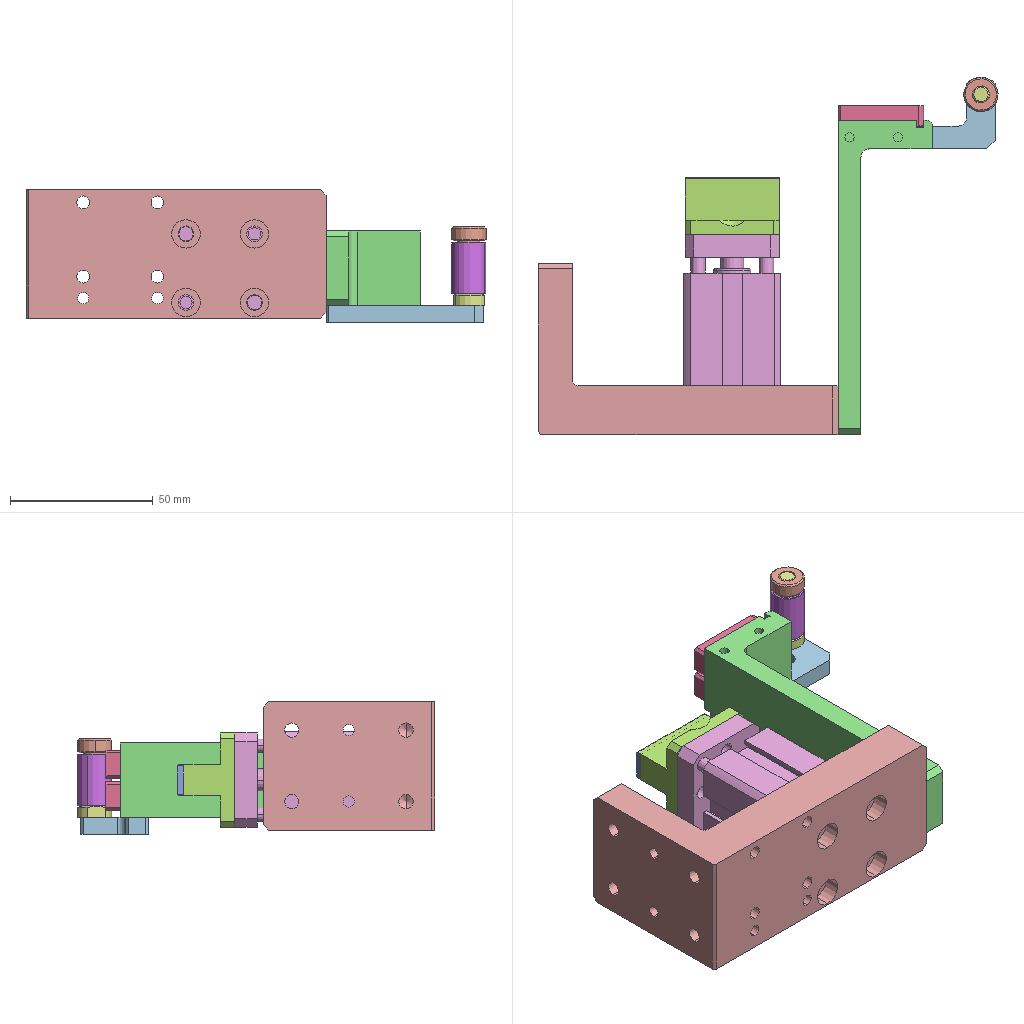Assembly | SolidWorks | 14 different items | 18 placed | box 161 x 125 x 46 mm
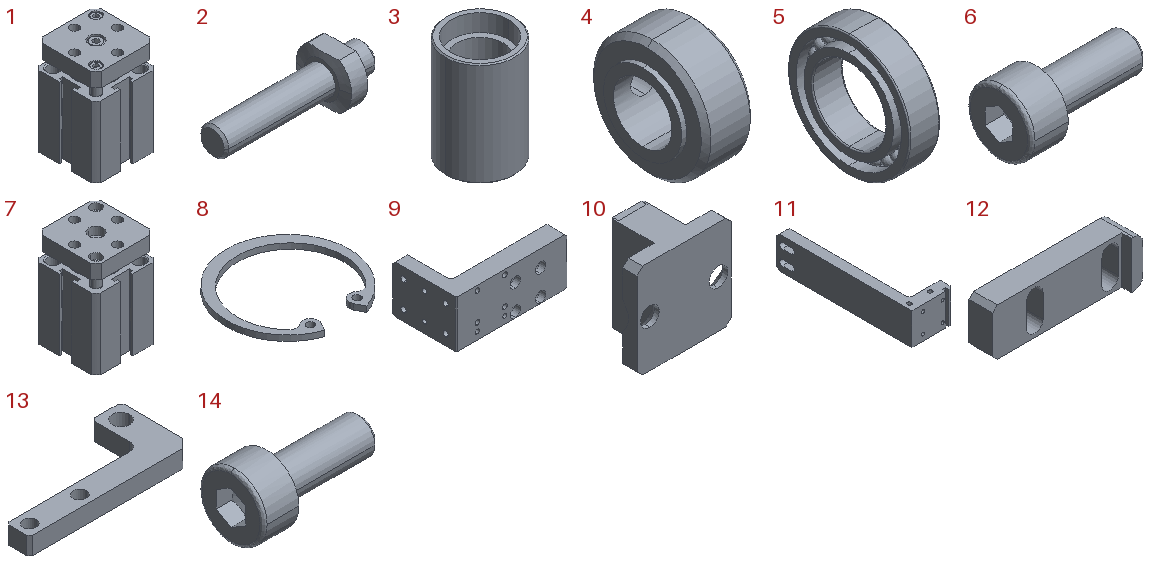Parts list (item | name | quantity | parent item | size | volume | features):
1 | (subassembly) | x1 | - | 34 x 34 x 53 mm | 43812 mm3 | -
2 | - | x1 | - | 32.5 x 12 x 10 mm | 1165 mm3 | features Chamfer 1, HoleWzd 1, ICE 1, Revolution 1
3 | - | x1 | - | 12 x 12 x 18 mm | 959.836 mm3 | features Chamfer 1, Extrusion 1, ICE 1, MirrorPattern 1
4 | - | x1 | - | 5.5 x 12 x 12 mm | 411.056 mm3 | features Chamfer 1, HoleWzd 1, Revolution 1
5 | - | x2 | - | 2.5 x 10 x 10 mm | 92.163 mm3 | features Stock 1
6 | - | x1 | in 1 | 14 x 7 x 7 mm | 259.154 mm3 | features BaseBody 1
7 | - | x1 | in 1 | 34 x 34 x 53 mm | 43056 mm3 | features BaseBody 1
8 | - | x2 | in 1 | 24.35 x 23.625 x 1.1 mm | 130.198 mm3 | features BaseBody 1
9 | - | x1 | - | 105 x 60 x 45 mm | 97512 mm3 | features HoleWzd 6, Chamfer 2, Extrusion 1, Fillet 1
10 | - | x1 | - | 33 x 20 x 33 mm | 10213 mm3 | features ICE 2, Chamfer 1, Extrusion 1, HoleWzd 1
11 | - | x1 | - | 33 x 110 x 26 mm | 27890 mm3 | features Fillet 2, HoleWzd 2, ICE 2, Chamfer 1, Extrusion 1, MirrorPattern 1
12 | - | x2 | - | 30 x 7 x 10 mm | 1262 mm3 | features Chamfer 1, Extrusion 1, Fillet 1, ICE 1
13 | - | x1 | - | 55 x 24 x 6 mm | 3212 mm3 | features Chamfer 2, Extrusion 1, Fillet 1
14 | - | x2 | in 1 | 11 x 5.5 x 5.5 mm | 118.284 mm3 | features BaseBody 1
Mates (type | each side: item.copy, entity, surface, feature):
Coincident | 10.1 face plane Boss-Extrude1 | 7.1 face plane Input 1
Concentric | 10.1 face cylinder Hole size per cross recess wood screw type 1 | 7.1 face cylinder Input 1 | 2 times
Coincident | 9.1 face plane Boss-Extrude1 | 7.1 face plane Input 1
Concentric | 9.1 face cylinder Hole size per socket head cap screw type 1 | 7.1 face cylinder Input 1 | 2 times
Coincident | 11.1 face plane Boss-Extrude1 | 13.1 face plane Boss-Extrude1
Concentric | 11.1 face cylinder M4 Tapped Hole1 | 13.1 face cylinder Boss-Extrude1 | 2 times
Coincident | 11.1 face plane Boss-Extrude1 | 12.1 face plane Boss-Extrude1
Coincident | 11.1 face plane Boss-Extrude1 | 12.2 face plane Boss-Extrude1
Concentric | 11.1 face cylinder M3 Tapped Hole1 | 12.1 face cylinder Cut-Extrude1 | 2 times
Concentric | 11.1 face cylinder M3 Tapped Hole1 | 12.2 face cylinder Cut-Extrude1 | 2 times
Coincident | 13.1 face plane Boss-Extrude1 | 2.1 face plane Revolve1
Concentric | 13.1 face cylinder Boss-Extrude1 | 2.1 face cylinder Revolve1
Coincident | 9.1 face plane Boss-Extrude1 | 11.1 face plane Boss-Extrude1 | 2 times
DistanceDim | 11.1 face plane Cut-Extrude2 | 9.1 face cylinder M4 Tapped Hole1
Concentric | 2.1 face cylinder Revolve1 | 5.1 face cylinder deep groove ball bearings gb
Coincident | 2.1 face plane Revolve1 | 5.1 face plane deep groove ball bearings gb
Coincident | 3.1 edge | 5.2 face cylinder deep groove ball bearings gb
Concentric | 3.1 face cylinder Boss-Extrude1 | 5.1 face cylinder deep groove ball bearings gb
Coincident | 3.1 face plane Boss-Extrude1 | 5.2 face plane deep groove ball bearings gb
Concentric | 2.1 face cylinder Revolve1 | 4.1 face cylinder Revolve1
Coincident | 5.2 face plane deep groove ball bearings gb | 4.1 face plane Revolve1
Coincident | 3.1 face plane Boss-Extrude1 | 5.1 face plane deep groove ball bearings gb